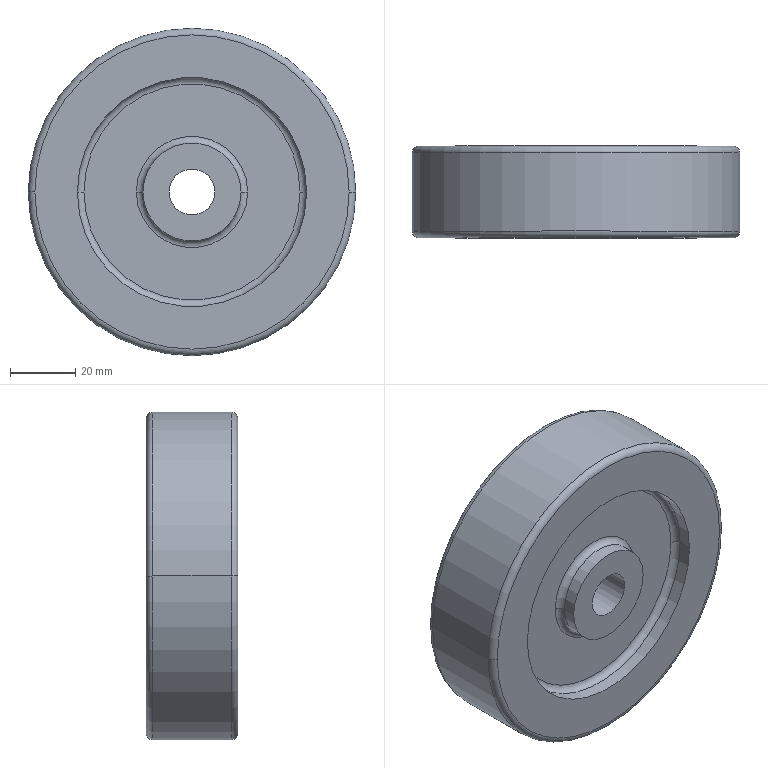Part | SolidWorks | features Fillet 2, Revolution 1 | 1 solid | 30 faces | box 100 x 28 x 100 mm | volume 177907 mm3 | torus 12 | cylinder 12 | plane 6 | commonest cylinder face diameters 30 x4 70 x4 14 x2 100 x2
STEP:
#1=CARTESIAN_POINT('',(-50.,-12.,0.));
#2=VERTEX_POINT('',#1);
#3=CARTESIAN_POINT('',(50.,-12.,0.));
#4=VERTEX_POINT('',#3);
#5=CARTESIAN_POINT('',(0.,-12.,0.));
#6=DIRECTION('',(0.,1.,0.));
#7=DIRECTION('',(1.,0.,0.));
#8=AXIS2_PLACEMENT_3D('',#5,#6,#7);
#9=CIRCLE('',#8,50.);
#10=EDGE_CURVE('',#2,#4,#9,.T.);
#11=ORIENTED_EDGE('',*,*,#10,.F.);
#12=CARTESIAN_POINT('',(-48.,-14.,0.));
#13=VERTEX_POINT('',#12);
#14=CARTESIAN_POINT('',(-48.,-12.,0.));
#15=DIRECTION('',(0.,0.,1.));
#16=DIRECTION('',(1.,0.,0.));
#17=AXIS2_PLACEMENT_3D('',#14,#15,#16);
#18=CIRCLE('',#17,2.);
#19=EDGE_CURVE('',#2,#13,#18,.T.);
#20=ORIENTED_EDGE('',*,*,#19,.T.);
#21=CARTESIAN_POINT('',(48.,-14.,0.));
#22=VERTEX_POINT('',#21);
#23=CARTESIAN_POINT('',(0.,-14.,0.));
#24=DIRECTION('',(0.,-1.,0.));
#25=DIRECTION('',(1.,0.,0.));
#26=AXIS2_PLACEMENT_3D('',#23,#24,#25);
#27=CIRCLE('',#26,48.);
#28=EDGE_CURVE('',#22,#13,#27,.T.);
#29=ORIENTED_EDGE('',*,*,#28,.F.);
#30=CARTESIAN_POINT('',(48.,-12.,0.));
#31=DIRECTION('',(0.,0.,-1.));
#32=DIRECTION('',(-1.,0.,0.));
#33=AXIS2_PLACEMENT_3D('',#30,#31,#32);
#34=CIRCLE('',#33,2.);
#35=EDGE_CURVE('',#4,#22,#34,.T.);
#36=ORIENTED_EDGE('',*,*,#35,.F.);
#37=EDGE_LOOP('',(#11,#20,#29,#36));
#38=FACE_OUTER_BOUND('',#37,.T.);
#39=CARTESIAN_POINT('',(0.,-12.,0.));
#40=DIRECTION('',(0.,-1.,0.));
#41=DIRECTION('',(1.,0.,0.));
#42=AXIS2_PLACEMENT_3D('',#39,#40,#41);
#43=TOROIDAL_SURFACE('',#42,48.,2.);
#44=ADVANCED_FACE('',(#38),#43,.T.);
#45=CARTESIAN_POINT('',(-33.,-8.,0.));
#46=VERTEX_POINT('',#45);
#47=CARTESIAN_POINT('',(33.,-8.,0.));
#48=VERTEX_POINT('',#47);
#49=CARTESIAN_POINT('',(0.,-8.,0.));
#50=DIRECTION('',(0.,-1.,0.));
#51=DIRECTION('',(1.,0.,0.));
#52=AXIS2_PLACEMENT_3D('',#49,#50,#51);
#53=CIRCLE('',#52,33.);
#54=EDGE_CURVE('',#46,#48,#53,.T.);
#55=ORIENTED_EDGE('',*,*,#54,.F.);
#56=CARTESIAN_POINT('',(-35.,-10.,0.));
#57=VERTEX_POINT('',#56);
#58=CARTESIAN_POINT('',(-33.,-10.,0.));
#59=DIRECTION('',(0.,0.,1.));
#60=DIRECTION('',(1.,0.,0.));
#61=AXIS2_PLACEMENT_3D('',#58,#59,#60);
#62=CIRCLE('',#61,2.);
#63=EDGE_CURVE('',#46,#57,#62,.T.);
#64=ORIENTED_EDGE('',*,*,#63,.T.);
#65=CARTESIAN_POINT('',(35.,-10.,0.));
#66=VERTEX_POINT('',#65);
#67=CARTESIAN_POINT('',(0.,-10.,0.));
#68=DIRECTION('',(0.,1.,0.));
#69=DIRECTION('',(1.,0.,0.));
#70=AXIS2_PLACEMENT_3D('',#67,#68,#69);
#71=CIRCLE('',#70,35.);
#72=EDGE_CURVE('',#66,#57,#71,.T.);
#73=ORIENTED_EDGE('',*,*,#72,.F.);
#74=CARTESIAN_POINT('',(33.,-10.,0.));
#75=DIRECTION('',(0.,0.,-1.));
#76=DIRECTION('',(-1.,0.,0.));
#77=AXIS2_PLACEMENT_3D('',#74,#75,#76);
#78=CIRCLE('',#77,2.);
#79=EDGE_CURVE('',#48,#66,#78,.T.);
#80=ORIENTED_EDGE('',*,*,#79,.F.);
#81=EDGE_LOOP('',(#55,#64,#73,#80));
#82=FACE_OUTER_BOUND('',#81,.T.);
#83=CARTESIAN_POINT('',(0.,-10.,0.));
#84=DIRECTION('',(0.,-1.,0.));
#85=DIRECTION('',(1.,0.,0.));
#86=AXIS2_PLACEMENT_3D('',#83,#84,#85);
#87=TOROIDAL_SURFACE('',#86,33.,2.);
#88=ADVANCED_FACE('',(#82),#87,.F.);
#89=CARTESIAN_POINT('',(-15.,-10.,0.));
#90=VERTEX_POINT('',#89);
#91=CARTESIAN_POINT('',(15.,-10.,0.));
#92=VERTEX_POINT('',#91);
#93=CARTESIAN_POINT('',(0.,-10.,0.));
#94=DIRECTION('',(0.,-1.,0.));
#95=DIRECTION('',(1.,0.,0.));
#96=AXIS2_PLACEMENT_3D('',#93,#94,#95);
#97=CIRCLE('',#96,15.);
#98=EDGE_CURVE('',#90,#92,#97,.T.);
#99=ORIENTED_EDGE('',*,*,#98,.F.);
#100=CARTESIAN_POINT('',(-17.,-8.,0.));
#101=VERTEX_POINT('',#100);
#102=CARTESIAN_POINT('',(-17.,-10.,0.));
#103=DIRECTION('',(0.,0.,1.));
#104=DIRECTION('',(1.,0.,0.));
#105=AXIS2_PLACEMENT_3D('',#102,#103,#104);
#106=CIRCLE('',#105,2.);
#107=EDGE_CURVE('',#90,#101,#106,.T.);
#108=ORIENTED_EDGE('',*,*,#107,.T.);
#109=CARTESIAN_POINT('',(17.,-8.,0.));
#110=VERTEX_POINT('',#109);
#111=CARTESIAN_POINT('',(0.,-8.,0.));
#112=DIRECTION('',(0.,1.,0.));
#113=DIRECTION('',(1.,0.,0.));
#114=AXIS2_PLACEMENT_3D('',#111,#112,#113);
#115=CIRCLE('',#114,17.);
#116=EDGE_CURVE('',#110,#101,#115,.T.);
#117=ORIENTED_EDGE('',*,*,#116,.F.);
#118=CARTESIAN_POINT('',(17.,-10.,0.));
#119=DIRECTION('',(0.,0.,-1.));
#120=DIRECTION('',(-1.,0.,0.));
#121=AXIS2_PLACEMENT_3D('',#118,#119,#120);
#122=CIRCLE('',#121,2.);
#123=EDGE_CURVE('',#92,#110,#122,.T.);
#124=ORIENTED_EDGE('',*,*,#123,.F.);
#125=EDGE_LOOP('',(#99,#108,#117,#124));
#126=FACE_OUTER_BOUND('',#125,.T.);
#127=CARTESIAN_POINT('',(0.,-10.,0.));
#128=DIRECTION('',(0.,-1.,0.));
#129=DIRECTION('',(1.,0.,0.));
#130=AXIS2_PLACEMENT_3D('',#127,#128,#129);
#131=TOROIDAL_SURFACE('',#130,17.,2.);
#132=ADVANCED_FACE('',(#126),#131,.F.);
#133=CARTESIAN_POINT('',(15.,10.,0.));
#134=VERTEX_POINT('',#133);
#135=CARTESIAN_POINT('',(-15.,10.,0.));
#136=VERTEX_POINT('',#135);
#137=CARTESIAN_POINT('',(0.,10.,0.));
#138=DIRECTION('',(0.,1.,0.));
#139=DIRECTION('',(-1.,0.,0.));
#140=AXIS2_PLACEMENT_3D('',#137,#138,#139);
#141=CIRCLE('',#140,15.);
#142=EDGE_CURVE('',#134,#136,#141,.T.);
#143=ORIENTED_EDGE('',*,*,#142,.F.);
#144=CARTESIAN_POINT('',(17.,8.,0.));
#145=VERTEX_POINT('',#144);
#146=CARTESIAN_POINT('',(17.,10.,0.));
#147=DIRECTION('',(0.,0.,1.));
#148=DIRECTION('',(1.,0.,0.));
#149=AXIS2_PLACEMENT_3D('',#146,#147,#148);
#150=CIRCLE('',#149,2.);
#151=EDGE_CURVE('',#134,#145,#150,.T.);
#152=ORIENTED_EDGE('',*,*,#151,.T.);
#153=CARTESIAN_POINT('',(-17.,8.,0.));
#154=VERTEX_POINT('',#153);
#155=CARTESIAN_POINT('',(0.,8.,0.));
#156=DIRECTION('',(0.,-1.,0.));
#157=DIRECTION('',(-1.,0.,0.));
#158=AXIS2_PLACEMENT_3D('',#155,#156,#157);
#159=CIRCLE('',#158,17.);
#160=EDGE_CURVE('',#154,#145,#159,.T.);
#161=ORIENTED_EDGE('',*,*,#160,.F.);
#162=CARTESIAN_POINT('',(-17.,10.,0.));
#163=DIRECTION('',(0.,0.,-1.));
#164=DIRECTION('',(-1.,0.,0.));
#165=AXIS2_PLACEMENT_3D('',#162,#163,#164);
#166=CIRCLE('',#165,2.);
#167=EDGE_CURVE('',#136,#154,#166,.T.);
#168=ORIENTED_EDGE('',*,*,#167,.F.);
#169=EDGE_LOOP('',(#143,#152,#161,#168));
#170=FACE_OUTER_BOUND('',#169,.T.);
#171=CARTESIAN_POINT('',(0.,10.,0.));
#172=DIRECTION('',(0.,1.,0.));
#173=DIRECTION('',(-1.,0.,0.));
#174=AXIS2_PLACEMENT_3D('',#171,#172,#173);
#175=TOROIDAL_SURFACE('',#174,17.,2.);
#176=ADVANCED_FACE('',(#170),#175,.F.);
#177=CARTESIAN_POINT('',(33.,8.,0.));
#178=VERTEX_POINT('',#177);
#179=CARTESIAN_POINT('',(-33.,8.,0.));
#180=VERTEX_POINT('',#179);
#181=CARTESIAN_POINT('',(0.,8.,0.));
#182=DIRECTION('',(0.,1.,0.));
#183=DIRECTION('',(-1.,0.,0.));
#184=AXIS2_PLACEMENT_3D('',#181,#182,#183);
#185=CIRCLE('',#184,33.);
#186=EDGE_CURVE('',#178,#180,#185,.T.);
#187=ORIENTED_EDGE('',*,*,#186,.F.);
#188=CARTESIAN_POINT('',(35.,10.,0.));
#189=VERTEX_POINT('',#188);
#190=CARTESIAN_POINT('',(33.,10.,0.));
#191=DIRECTION('',(0.,0.,1.));
#192=DIRECTION('',(1.,0.,0.));
#193=AXIS2_PLACEMENT_3D('',#190,#191,#192);
#194=CIRCLE('',#193,2.);
#195=EDGE_CURVE('',#178,#189,#194,.T.);
#196=ORIENTED_EDGE('',*,*,#195,.T.);
#197=CARTESIAN_POINT('',(-35.,10.,0.));
#198=VERTEX_POINT('',#197);
#199=CARTESIAN_POINT('',(0.,10.,0.));
#200=DIRECTION('',(0.,-1.,0.));
#201=DIRECTION('',(-1.,0.,0.));
#202=AXIS2_PLACEMENT_3D('',#199,#200,#201);
#203=CIRCLE('',#202,35.);
#204=EDGE_CURVE('',#198,#189,#203,.T.);
#205=ORIENTED_EDGE('',*,*,#204,.F.);
#206=CARTESIAN_POINT('',(-33.,10.,0.));
#207=DIRECTION('',(0.,0.,-1.));
#208=DIRECTION('',(-1.,0.,0.));
#209=AXIS2_PLACEMENT_3D('',#206,#207,#208);
#210=CIRCLE('',#209,2.);
#211=EDGE_CURVE('',#180,#198,#210,.T.);
#212=ORIENTED_EDGE('',*,*,#211,.F.);
#213=EDGE_LOOP('',(#187,#196,#205,#212));
#214=FACE_OUTER_BOUND('',#213,.T.);
#215=CARTESIAN_POINT('',(0.,10.,0.));
#216=DIRECTION('',(0.,1.,0.));
#217=DIRECTION('',(-1.,0.,0.));
#218=AXIS2_PLACEMENT_3D('',#215,#216,#217);
#219=TOROIDAL_SURFACE('',#218,33.,2.);
#220=ADVANCED_FACE('',(#214),#219,.F.);
#221=CARTESIAN_POINT('',(50.,12.,0.));
#222=VERTEX_POINT('',#221);
#223=CARTESIAN_POINT('',(-50.,12.,0.));
#224=VERTEX_POINT('',#223);
#225=CARTESIAN_POINT('',(0.,12.,0.));
#226=DIRECTION('',(0.,-1.,0.));
#227=DIRECTION('',(-1.,0.,0.));
#228=AXIS2_PLACEMENT_3D('',#225,#226,#227);
#229=CIRCLE('',#228,50.);
#230=EDGE_CURVE('',#222,#224,#229,.T.);
#231=ORIENTED_EDGE('',*,*,#230,.F.);
#232=CARTESIAN_POINT('',(48.,14.,0.));
#233=VERTEX_POINT('',#232);
#234=CARTESIAN_POINT('',(48.,12.,0.));
#235=DIRECTION('',(0.,0.,1.));
#236=DIRECTION('',(1.,0.,0.));
#237=AXIS2_PLACEMENT_3D('',#234,#235,#236);
#238=CIRCLE('',#237,2.);
#239=EDGE_CURVE('',#222,#233,#238,.T.);
#240=ORIENTED_EDGE('',*,*,#239,.T.);
#241=CARTESIAN_POINT('',(-48.,14.,0.));
#242=VERTEX_POINT('',#241);
#243=CARTESIAN_POINT('',(0.,14.,0.));
#244=DIRECTION('',(0.,1.,0.));
#245=DIRECTION('',(-1.,0.,0.));
#246=AXIS2_PLACEMENT_3D('',#243,#244,#245);
#247=CIRCLE('',#246,48.);
#248=EDGE_CURVE('',#242,#233,#247,.T.);
#249=ORIENTED_EDGE('',*,*,#248,.F.);
#250=CARTESIAN_POINT('',(-48.,12.,0.));
#251=DIRECTION('',(0.,0.,-1.));
#252=DIRECTION('',(-1.,0.,0.));
#253=AXIS2_PLACEMENT_3D('',#250,#251,#252);
#254=CIRCLE('',#253,2.);
#255=EDGE_CURVE('',#224,#242,#254,.T.);
#256=ORIENTED_EDGE('',*,*,#255,.F.);
#257=EDGE_LOOP('',(#231,#240,#249,#256));
#258=FACE_OUTER_BOUND('',#257,.T.);
#259=CARTESIAN_POINT('',(0.,12.,0.));
#260=DIRECTION('',(0.,1.,0.));
#261=DIRECTION('',(-1.,0.,0.));
#262=AXIS2_PLACEMENT_3D('',#259,#260,#261);
#263=TOROIDAL_SURFACE('',#262,48.,2.);
#264=ADVANCED_FACE('',(#258),#263,.T.);
#265=CARTESIAN_POINT('',(-7.,14.,0.));
#266=VERTEX_POINT('',#265);
#267=CARTESIAN_POINT('',(7.,14.,0.));
#268=VERTEX_POINT('',#267);
#269=CARTESIAN_POINT('',(0.,14.,0.));
#270=DIRECTION('',(0.,-1.,0.));
#271=DIRECTION('',(1.,0.,0.));
#272=AXIS2_PLACEMENT_3D('',#269,#270,#271);
#273=CIRCLE('',#272,7.);
#274=EDGE_CURVE('',#266,#268,#273,.T.);
#275=ORIENTED_EDGE('',*,*,#274,.F.);
#276=CARTESIAN_POINT('',(-7.,-14.,0.));
#277=VERTEX_POINT('',#276);
#278=CARTESIAN_POINT('',(-7.,-499.995,0.));
#279=DIRECTION('',(0.,-1.,0.));
#280=VECTOR('',#279,1000.);
#281=LINE('',#278,#280);
#282=EDGE_CURVE('',#266,#277,#281,.T.);
#283=ORIENTED_EDGE('',*,*,#282,.T.);
#284=CARTESIAN_POINT('',(7.,-14.,0.));
#285=VERTEX_POINT('',#284);
#286=CARTESIAN_POINT('',(0.,-14.,0.));
#287=DIRECTION('',(0.,-1.,0.));
#288=DIRECTION('',(1.,0.,0.));
#289=AXIS2_PLACEMENT_3D('',#286,#287,#288);
#290=CIRCLE('',#289,7.);
#291=EDGE_CURVE('',#277,#285,#290,.T.);
#292=ORIENTED_EDGE('',*,*,#291,.T.);
#293=CARTESIAN_POINT('',(7.,-499.995,0.));
#294=DIRECTION('',(0.,-1.,0.));
#295=VECTOR('',#294,1000.);
#296=LINE('',#293,#295);
#297=EDGE_CURVE('',#268,#285,#296,.T.);
#298=ORIENTED_EDGE('',*,*,#297,.F.);
#299=EDGE_LOOP('',(#275,#283,#292,#298));
#300=FACE_OUTER_BOUND('',#299,.T.);
#301=CARTESIAN_POINT('',(0.,-499.995,0.));
#302=DIRECTION('',(0.,-1.,0.));
#303=DIRECTION('',(1.,0.,0.));
#304=AXIS2_PLACEMENT_3D('',#301,#302,#303);
#305=CYLINDRICAL_SURFACE('',#304,7.);
#306=ADVANCED_FACE('',(#300),#305,.F.);
#307=CARTESIAN_POINT('',(15.,14.,0.));
#308=VERTEX_POINT('',#307);
#309=CARTESIAN_POINT('',(-15.,14.,0.));
#310=VERTEX_POINT('',#309);
#311=CARTESIAN_POINT('',(0.,14.,0.));
#312=DIRECTION('',(0.,-1.,0.));
#313=DIRECTION('',(1.,0.,0.));
#314=AXIS2_PLACEMENT_3D('',#311,#312,#313);
#315=CIRCLE('',#314,15.);
#316=EDGE_CURVE('',#308,#310,#315,.T.);
#317=ORIENTED_EDGE('',*,*,#316,.T.);
#318=CARTESIAN_POINT('',(-15.,-499.995,0.));
#319=DIRECTION('',(0.,-1.,0.));
#320=VECTOR('',#319,1000.);
#321=LINE('',#318,#320);
#322=EDGE_CURVE('',#310,#136,#321,.T.);
#323=ORIENTED_EDGE('',*,*,#322,.T.);
#324=CARTESIAN_POINT('',(0.,10.,0.));
#325=DIRECTION('',(0.,1.,0.));
#326=DIRECTION('',(-1.,0.,0.));
#327=AXIS2_PLACEMENT_3D('',#324,#325,#326);
#328=CIRCLE('',#327,15.);
#329=EDGE_CURVE('',#136,#134,#328,.T.);
#330=ORIENTED_EDGE('',*,*,#329,.T.);
#331=CARTESIAN_POINT('',(15.,-499.995,0.));
#332=DIRECTION('',(0.,-1.,0.));
#333=VECTOR('',#332,1000.);
#334=LINE('',#331,#333);
#335=EDGE_CURVE('',#308,#134,#334,.T.);
#336=ORIENTED_EDGE('',*,*,#335,.F.);
#337=EDGE_LOOP('',(#317,#323,#330,#336));
#338=FACE_OUTER_BOUND('',#337,.T.);
#339=CARTESIAN_POINT('',(0.,-499.995,0.));
#340=DIRECTION('',(0.,-1.,0.));
#341=DIRECTION('',(1.,0.,0.));
#342=AXIS2_PLACEMENT_3D('',#339,#340,#341);
#343=CYLINDRICAL_SURFACE('',#342,15.);
#344=ADVANCED_FACE('',(#338),#343,.T.);
#345=CARTESIAN_POINT('',(-35.,14.,0.));
#346=VERTEX_POINT('',#345);
#347=CARTESIAN_POINT('',(35.,14.,0.));
#348=VERTEX_POINT('',#347);
#349=CARTESIAN_POINT('',(0.,14.,0.));
#350=DIRECTION('',(0.,-1.,0.));
#351=DIRECTION('',(1.,0.,0.));
#352=AXIS2_PLACEMENT_3D('',#349,#350,#351);
#353=CIRCLE('',#352,35.);
#354=EDGE_CURVE('',#346,#348,#353,.T.);
#355=ORIENTED_EDGE('',*,*,#354,.F.);
#356=CARTESIAN_POINT('',(-35.,-499.995,0.));
#357=DIRECTION('',(0.,-1.,0.));
#358=VECTOR('',#357,1000.);
#359=LINE('',#356,#358);
#360=EDGE_CURVE('',#346,#198,#359,.T.);
#361=ORIENTED_EDGE('',*,*,#360,.T.);
#362=ORIENTED_EDGE('',*,*,#204,.T.);
#363=CARTESIAN_POINT('',(35.,-499.995,0.));
#364=DIRECTION('',(0.,-1.,0.));
#365=VECTOR('',#364,1000.);
#366=LINE('',#363,#365);
#367=EDGE_CURVE('',#348,#189,#366,.T.);
#368=ORIENTED_EDGE('',*,*,#367,.F.);
#369=EDGE_LOOP('',(#355,#361,#362,#368));
#370=FACE_OUTER_BOUND('',#369,.T.);
#371=CARTESIAN_POINT('',(0.,-499.995,0.));
#372=DIRECTION('',(0.,-1.,0.));
#373=DIRECTION('',(1.,0.,0.));
#374=AXIS2_PLACEMENT_3D('',#371,#372,#373);
#375=CYLINDRICAL_SURFACE('',#374,35.);
#376=ADVANCED_FACE('',(#370),#375,.F.);
#377=ORIENTED_EDGE('',*,*,#230,.T.);
#378=CARTESIAN_POINT('',(-50.,-499.995,0.));
#379=DIRECTION('',(0.,-1.,0.));
#380=VECTOR('',#379,1000.);
#381=LINE('',#378,#380);
#382=EDGE_CURVE('',#224,#2,#381,.T.);
#383=ORIENTED_EDGE('',*,*,#382,.T.);
#384=ORIENTED_EDGE('',*,*,#10,.T.);
#385=CARTESIAN_POINT('',(50.,-499.995,0.));
#386=DIRECTION('',(0.,-1.,0.));
#387=VECTOR('',#386,1000.);
#388=LINE('',#385,#387);
#389=EDGE_CURVE('',#222,#4,#388,.T.);
#390=ORIENTED_EDGE('',*,*,#389,.F.);
#391=EDGE_LOOP('',(#377,#383,#384,#390));
#392=FACE_OUTER_BOUND('',#391,.T.);
#393=CARTESIAN_POINT('',(0.,-499.995,0.));
#394=DIRECTION('',(0.,-1.,0.));
#395=DIRECTION('',(1.,0.,0.));
#396=AXIS2_PLACEMENT_3D('',#393,#394,#395);
#397=CYLINDRICAL_SURFACE('',#396,50.);
#398=ADVANCED_FACE('',(#392),#397,.T.);
#399=ORIENTED_EDGE('',*,*,#72,.T.);
#400=CARTESIAN_POINT('',(-35.,-14.,0.));
#401=VERTEX_POINT('',#400);
#402=CARTESIAN_POINT('',(-35.,-499.995,0.));
#403=DIRECTION('',(0.,-1.,0.));
#404=VECTOR('',#403,1000.);
#405=LINE('',#402,#404);
#406=EDGE_CURVE('',#57,#401,#405,.T.);
#407=ORIENTED_EDGE('',*,*,#406,.T.);
#408=CARTESIAN_POINT('',(35.,-14.,0.));
#409=VERTEX_POINT('',#408);
#410=CARTESIAN_POINT('',(0.,-14.,0.));
#411=DIRECTION('',(0.,-1.,0.));
#412=DIRECTION('',(1.,0.,0.));
#413=AXIS2_PLACEMENT_3D('',#410,#411,#412);
#414=CIRCLE('',#413,35.);
#415=EDGE_CURVE('',#401,#409,#414,.T.);
#416=ORIENTED_EDGE('',*,*,#415,.T.);
#417=CARTESIAN_POINT('',(35.,-499.995,0.));
#418=DIRECTION('',(0.,-1.,0.));
#419=VECTOR('',#418,1000.);
#420=LINE('',#417,#419);
#421=EDGE_CURVE('',#66,#409,#420,.T.);
#422=ORIENTED_EDGE('',*,*,#421,.F.);
#423=EDGE_LOOP('',(#399,#407,#416,#422));
#424=FACE_OUTER_BOUND('',#423,.T.);
#425=CARTESIAN_POINT('',(0.,-499.995,0.));
#426=DIRECTION('',(0.,-1.,0.));
#427=DIRECTION('',(1.,0.,0.));
#428=AXIS2_PLACEMENT_3D('',#425,#426,#427);
#429=CYLINDRICAL_SURFACE('',#428,35.);
#430=ADVANCED_FACE('',(#424),#429,.F.);
#431=CARTESIAN_POINT('',(0.,-10.,0.));
#432=DIRECTION('',(0.,-1.,0.));
#433=DIRECTION('',(1.,0.,0.));
#434=AXIS2_PLACEMENT_3D('',#431,#432,#433);
#435=CIRCLE('',#434,15.);
#436=EDGE_CURVE('',#92,#90,#435,.T.);
#437=ORIENTED_EDGE('',*,*,#436,.T.);
#438=CARTESIAN_POINT('',(-15.,-14.,0.));
#439=VERTEX_POINT('',#438);
#440=CARTESIAN_POINT('',(-15.,-499.995,0.));
#441=DIRECTION('',(0.,-1.,0.));
#442=VECTOR('',#441,1000.);
#443=LINE('',#440,#442);
#444=EDGE_CURVE('',#90,#439,#443,.T.);
#445=ORIENTED_EDGE('',*,*,#444,.T.);
#446=CARTESIAN_POINT('',(15.,-14.,0.));
#447=VERTEX_POINT('',#446);
#448=CARTESIAN_POINT('',(0.,-14.,0.));
#449=DIRECTION('',(0.,-1.,0.));
#450=DIRECTION('',(1.,0.,0.));
#451=AXIS2_PLACEMENT_3D('',#448,#449,#450);
#452=CIRCLE('',#451,15.);
#453=EDGE_CURVE('',#447,#439,#452,.T.);
#454=ORIENTED_EDGE('',*,*,#453,.F.);
#455=CARTESIAN_POINT('',(15.,-499.995,0.));
#456=DIRECTION('',(0.,-1.,0.));
#457=VECTOR('',#456,1000.);
#458=LINE('',#455,#457);
#459=EDGE_CURVE('',#92,#447,#458,.T.);
#460=ORIENTED_EDGE('',*,*,#459,.F.);
#461=EDGE_LOOP('',(#437,#445,#454,#460));
#462=FACE_OUTER_BOUND('',#461,.T.);
#463=CARTESIAN_POINT('',(0.,-499.995,0.));
#464=DIRECTION('',(0.,-1.,0.));
#465=DIRECTION('',(1.,0.,0.));
#466=AXIS2_PLACEMENT_3D('',#463,#464,#465);
#467=CYLINDRICAL_SURFACE('',#466,15.);
#468=ADVANCED_FACE('',(#462),#467,.T.);
#469=ORIENTED_EDGE('',*,*,#444,.F.);
#470=ORIENTED_EDGE('',*,*,#98,.T.);
#471=ORIENTED_EDGE('',*,*,#459,.T.);
#472=CARTESIAN_POINT('',(0.,-14.,0.));
#473=DIRECTION('',(0.,-1.,0.));
#474=DIRECTION('',(1.,0.,0.));
#475=AXIS2_PLACEMENT_3D('',#472,#473,#474);
#476=CIRCLE('',#475,15.);
#477=EDGE_CURVE('',#439,#447,#476,.T.);
#478=ORIENTED_EDGE('',*,*,#477,.F.);
#479=EDGE_LOOP('',(#469,#470,#471,#478));
#480=FACE_OUTER_BOUND('',#479,.T.);
#481=CARTESIAN_POINT('',(0.,-499.995,0.));
#482=DIRECTION('',(0.,-1.,0.));
#483=DIRECTION('',(1.,0.,0.));
#484=AXIS2_PLACEMENT_3D('',#481,#482,#483);
#485=CYLINDRICAL_SURFACE('',#484,15.);
#486=ADVANCED_FACE('',(#480),#485,.T.);
#487=ORIENTED_EDGE('',*,*,#116,.T.);
#488=CARTESIAN_POINT('',(0.,-8.,0.));
#489=DIRECTION('',(0.,1.,0.));
#490=DIRECTION('',(1.,0.,0.));
#491=AXIS2_PLACEMENT_3D('',#488,#489,#490);
#492=CIRCLE('',#491,17.);
#493=EDGE_CURVE('',#101,#110,#492,.T.);
#494=ORIENTED_EDGE('',*,*,#493,.T.);
#495=EDGE_LOOP('',(#487,#494));
#496=FACE_BOUND('',#495,.T.);
#497=CARTESIAN_POINT('',(0.,-8.,0.));
#498=DIRECTION('',(0.,-1.,0.));
#499=DIRECTION('',(1.,0.,0.));
#500=AXIS2_PLACEMENT_3D('',#497,#498,#499);
#501=CIRCLE('',#500,33.);
#502=EDGE_CURVE('',#48,#46,#501,.T.);
#503=ORIENTED_EDGE('',*,*,#502,.T.);
#504=ORIENTED_EDGE('',*,*,#54,.T.);
#505=EDGE_LOOP('',(#503,#504));
#506=FACE_OUTER_BOUND('',#505,.T.);
#507=CARTESIAN_POINT('',(35.,-8.,0.));
#508=DIRECTION('',(0.,-1.,0.));
#509=DIRECTION('',(1.,0.,0.));
#510=AXIS2_PLACEMENT_3D('',#507,#508,#509);
#511=PLANE('',#510);
#512=ADVANCED_FACE('',(#496,#506),#511,.T.);
#513=ORIENTED_EDGE('',*,*,#406,.F.);
#514=CARTESIAN_POINT('',(0.,-10.,0.));
#515=DIRECTION('',(0.,1.,0.));
#516=DIRECTION('',(1.,0.,0.));
#517=AXIS2_PLACEMENT_3D('',#514,#515,#516);
#518=CIRCLE('',#517,35.);
#519=EDGE_CURVE('',#57,#66,#518,.T.);
#520=ORIENTED_EDGE('',*,*,#519,.T.);
#521=ORIENTED_EDGE('',*,*,#421,.T.);
#522=CARTESIAN_POINT('',(0.,-14.,0.));
#523=DIRECTION('',(0.,-1.,0.));
#524=DIRECTION('',(1.,0.,0.));
#525=AXIS2_PLACEMENT_3D('',#522,#523,#524);
#526=CIRCLE('',#525,35.);
#527=EDGE_CURVE('',#409,#401,#526,.T.);
#528=ORIENTED_EDGE('',*,*,#527,.T.);
#529=EDGE_LOOP('',(#513,#520,#521,#528));
#530=FACE_OUTER_BOUND('',#529,.T.);
#531=CARTESIAN_POINT('',(0.,-499.995,0.));
#532=DIRECTION('',(0.,-1.,0.));
#533=DIRECTION('',(1.,0.,0.));
#534=AXIS2_PLACEMENT_3D('',#531,#532,#533);
#535=CYLINDRICAL_SURFACE('',#534,35.);
#536=ADVANCED_FACE('',(#530),#535,.F.);
#537=ORIENTED_EDGE('',*,*,#28,.T.);
#538=CARTESIAN_POINT('',(0.,-14.,0.));
#539=DIRECTION('',(0.,-1.,0.));
#540=DIRECTION('',(1.,0.,0.));
#541=AXIS2_PLACEMENT_3D('',#538,#539,#540);
#542=CIRCLE('',#541,48.);
#543=EDGE_CURVE('',#13,#22,#542,.T.);
#544=ORIENTED_EDGE('',*,*,#543,.T.);
#545=EDGE_LOOP('',(#537,#544));
#546=FACE_OUTER_BOUND('',#545,.T.);
#547=ORIENTED_EDGE('',*,*,#527,.F.);
#548=ORIENTED_EDGE('',*,*,#415,.F.);
#549=EDGE_LOOP('',(#547,#548));
#550=FACE_BOUND('',#549,.T.);
#551=CARTESIAN_POINT('',(50.,-14.,0.));
#552=DIRECTION('',(0.,-1.,0.));
#553=DIRECTION('',(1.,0.,0.));
#554=AXIS2_PLACEMENT_3D('',#551,#552,#553);
#555=PLANE('',#554);
#556=ADVANCED_FACE('',(#546,#550),#555,.T.);
#557=ORIENTED_EDGE('',*,*,#382,.F.);
#558=CARTESIAN_POINT('',(0.,12.,0.));
#559=DIRECTION('',(0.,-1.,0.));
#560=DIRECTION('',(-1.,0.,0.));
#561=AXIS2_PLACEMENT_3D('',#558,#559,#560);
#562=CIRCLE('',#561,50.);
#563=EDGE_CURVE('',#224,#222,#562,.T.);
#564=ORIENTED_EDGE('',*,*,#563,.T.);
#565=ORIENTED_EDGE('',*,*,#389,.T.);
#566=CARTESIAN_POINT('',(0.,-12.,0.));
#567=DIRECTION('',(0.,1.,0.));
#568=DIRECTION('',(1.,0.,0.));
#569=AXIS2_PLACEMENT_3D('',#566,#567,#568);
#570=CIRCLE('',#569,50.);
#571=EDGE_CURVE('',#4,#2,#570,.T.);
#572=ORIENTED_EDGE('',*,*,#571,.T.);
#573=EDGE_LOOP('',(#557,#564,#565,#572));
#574=FACE_OUTER_BOUND('',#573,.T.);
#575=CARTESIAN_POINT('',(0.,-499.995,0.));
#576=DIRECTION('',(0.,-1.,0.));
#577=DIRECTION('',(1.,0.,0.));
#578=AXIS2_PLACEMENT_3D('',#575,#576,#577);
#579=CYLINDRICAL_SURFACE('',#578,50.);
#580=ADVANCED_FACE('',(#574),#579,.T.);
#581=ORIENTED_EDGE('',*,*,#248,.T.);
#582=CARTESIAN_POINT('',(0.,14.,0.));
#583=DIRECTION('',(0.,1.,0.));
#584=DIRECTION('',(-1.,0.,0.));
#585=AXIS2_PLACEMENT_3D('',#582,#583,#584);
#586=CIRCLE('',#585,48.);
#587=EDGE_CURVE('',#233,#242,#586,.T.);
#588=ORIENTED_EDGE('',*,*,#587,.T.);
#589=EDGE_LOOP('',(#581,#588));
#590=FACE_OUTER_BOUND('',#589,.T.);
#591=CARTESIAN_POINT('',(0.,14.,0.));
#592=DIRECTION('',(0.,-1.,0.));
#593=DIRECTION('',(1.,0.,0.));
#594=AXIS2_PLACEMENT_3D('',#591,#592,#593);
#595=CIRCLE('',#594,35.);
#596=EDGE_CURVE('',#348,#346,#595,.T.);
#597=ORIENTED_EDGE('',*,*,#596,.T.);
#598=ORIENTED_EDGE('',*,*,#354,.T.);
#599=EDGE_LOOP('',(#597,#598));
#600=FACE_BOUND('',#599,.T.);
#601=CARTESIAN_POINT('',(35.,14.,0.));
#602=DIRECTION('',(0.,1.,0.));
#603=DIRECTION('',(-1.,0.,0.));
#604=AXIS2_PLACEMENT_3D('',#601,#602,#603);
#605=PLANE('',#604);
#606=ADVANCED_FACE('',(#590,#600),#605,.T.);
#607=ORIENTED_EDGE('',*,*,#360,.F.);
#608=ORIENTED_EDGE('',*,*,#596,.F.);
#609=ORIENTED_EDGE('',*,*,#367,.T.);
#610=CARTESIAN_POINT('',(0.,10.,0.));
#611=DIRECTION('',(0.,-1.,0.));
#612=DIRECTION('',(-1.,0.,0.));
#613=AXIS2_PLACEMENT_3D('',#610,#611,#612);
#614=CIRCLE('',#613,35.);
#615=EDGE_CURVE('',#189,#198,#614,.T.);
#616=ORIENTED_EDGE('',*,*,#615,.T.);
#617=EDGE_LOOP('',(#607,#608,#609,#616));
#618=FACE_OUTER_BOUND('',#617,.T.);
#619=CARTESIAN_POINT('',(0.,-499.995,0.));
#620=DIRECTION('',(0.,-1.,0.));
#621=DIRECTION('',(1.,0.,0.));
#622=AXIS2_PLACEMENT_3D('',#619,#620,#621);
#623=CYLINDRICAL_SURFACE('',#622,35.);
#624=ADVANCED_FACE('',(#618),#623,.F.);
#625=CARTESIAN_POINT('',(0.,8.,0.));
#626=DIRECTION('',(0.,1.,0.));
#627=DIRECTION('',(-1.,0.,0.));
#628=AXIS2_PLACEMENT_3D('',#625,#626,#627);
#629=CIRCLE('',#628,33.);
#630=EDGE_CURVE('',#180,#178,#629,.T.);
#631=ORIENTED_EDGE('',*,*,#630,.T.);
#632=ORIENTED_EDGE('',*,*,#186,.T.);
#633=EDGE_LOOP('',(#631,#632));
#634=FACE_OUTER_BOUND('',#633,.T.);
#635=ORIENTED_EDGE('',*,*,#160,.T.);
#636=CARTESIAN_POINT('',(0.,8.,0.));
#637=DIRECTION('',(0.,-1.,0.));
#638=DIRECTION('',(-1.,0.,0.));
#639=AXIS2_PLACEMENT_3D('',#636,#637,#638);
#640=CIRCLE('',#639,17.);
#641=EDGE_CURVE('',#145,#154,#640,.T.);
#642=ORIENTED_EDGE('',*,*,#641,.T.);
#643=EDGE_LOOP('',(#635,#642));
#644=FACE_BOUND('',#643,.T.);
#645=CARTESIAN_POINT('',(15.,8.,0.));
#646=DIRECTION('',(0.,1.,0.));
#647=DIRECTION('',(-1.,0.,0.));
#648=AXIS2_PLACEMENT_3D('',#645,#646,#647);
#649=PLANE('',#648);
#650=ADVANCED_FACE('',(#634,#644),#649,.T.);
#651=ORIENTED_EDGE('',*,*,#322,.F.);
#652=CARTESIAN_POINT('',(0.,14.,0.));
#653=DIRECTION('',(0.,-1.,0.));
#654=DIRECTION('',(1.,0.,0.));
#655=AXIS2_PLACEMENT_3D('',#652,#653,#654);
#656=CIRCLE('',#655,15.);
#657=EDGE_CURVE('',#310,#308,#656,.T.);
#658=ORIENTED_EDGE('',*,*,#657,.T.);
#659=ORIENTED_EDGE('',*,*,#335,.T.);
#660=ORIENTED_EDGE('',*,*,#142,.T.);
#661=EDGE_LOOP('',(#651,#658,#659,#660));
#662=FACE_OUTER_BOUND('',#661,.T.);
#663=CARTESIAN_POINT('',(0.,-499.995,0.));
#664=DIRECTION('',(0.,-1.,0.));
#665=DIRECTION('',(1.,0.,0.));
#666=AXIS2_PLACEMENT_3D('',#663,#664,#665);
#667=CYLINDRICAL_SURFACE('',#666,15.);
#668=ADVANCED_FACE('',(#662),#667,.T.);
#669=CARTESIAN_POINT('',(0.,14.,0.));
#670=DIRECTION('',(0.,-1.,0.));
#671=DIRECTION('',(1.,0.,0.));
#672=AXIS2_PLACEMENT_3D('',#669,#670,#671);
#673=CIRCLE('',#672,7.);
#674=EDGE_CURVE('',#268,#266,#673,.T.);
#675=ORIENTED_EDGE('',*,*,#674,.T.);
#676=ORIENTED_EDGE('',*,*,#274,.T.);
#677=EDGE_LOOP('',(#675,#676));
#678=FACE_BOUND('',#677,.T.);
#679=ORIENTED_EDGE('',*,*,#316,.F.);
#680=ORIENTED_EDGE('',*,*,#657,.F.);
#681=EDGE_LOOP('',(#679,#680));
#682=FACE_OUTER_BOUND('',#681,.T.);
#683=CARTESIAN_POINT('',(7.,14.,0.));
#684=DIRECTION('',(0.,1.,0.));
#685=DIRECTION('',(-1.,0.,0.));
#686=AXIS2_PLACEMENT_3D('',#683,#684,#685);
#687=PLANE('',#686);
#688=ADVANCED_FACE('',(#678,#682),#687,.T.);
#689=ORIENTED_EDGE('',*,*,#282,.F.);
#690=ORIENTED_EDGE('',*,*,#674,.F.);
#691=ORIENTED_EDGE('',*,*,#297,.T.);
#692=CARTESIAN_POINT('',(0.,-14.,0.));
#693=DIRECTION('',(0.,-1.,0.));
#694=DIRECTION('',(1.,0.,0.));
#695=AXIS2_PLACEMENT_3D('',#692,#693,#694);
#696=CIRCLE('',#695,7.);
#697=EDGE_CURVE('',#285,#277,#696,.T.);
#698=ORIENTED_EDGE('',*,*,#697,.T.);
#699=EDGE_LOOP('',(#689,#690,#691,#698));
#700=FACE_OUTER_BOUND('',#699,.T.);
#701=CARTESIAN_POINT('',(0.,-499.995,0.));
#702=DIRECTION('',(0.,-1.,0.));
#703=DIRECTION('',(1.,0.,0.));
#704=AXIS2_PLACEMENT_3D('',#701,#702,#703);
#705=CYLINDRICAL_SURFACE('',#704,7.);
#706=ADVANCED_FACE('',(#700),#705,.F.);
#707=ORIENTED_EDGE('',*,*,#453,.T.);
#708=ORIENTED_EDGE('',*,*,#477,.T.);
#709=EDGE_LOOP('',(#707,#708));
#710=FACE_OUTER_BOUND('',#709,.T.);
#711=ORIENTED_EDGE('',*,*,#697,.F.);
#712=ORIENTED_EDGE('',*,*,#291,.F.);
#713=EDGE_LOOP('',(#711,#712));
#714=FACE_BOUND('',#713,.T.);
#715=CARTESIAN_POINT('',(7.,-14.,0.));
#716=DIRECTION('',(0.,-1.,0.));
#717=DIRECTION('',(1.,0.,0.));
#718=AXIS2_PLACEMENT_3D('',#715,#716,#717);
#719=PLANE('',#718);
#720=ADVANCED_FACE('',(#710,#714),#719,.T.);
#721=ORIENTED_EDGE('',*,*,#239,.F.);
#722=ORIENTED_EDGE('',*,*,#563,.F.);
#723=ORIENTED_EDGE('',*,*,#255,.T.);
#724=ORIENTED_EDGE('',*,*,#587,.F.);
#725=EDGE_LOOP('',(#721,#722,#723,#724));
#726=FACE_OUTER_BOUND('',#725,.T.);
#727=CARTESIAN_POINT('',(0.,12.,0.));
#728=DIRECTION('',(0.,1.,0.));
#729=DIRECTION('',(-1.,0.,0.));
#730=AXIS2_PLACEMENT_3D('',#727,#728,#729);
#731=TOROIDAL_SURFACE('',#730,48.,2.);
#732=ADVANCED_FACE('',(#726),#731,.T.);
#733=ORIENTED_EDGE('',*,*,#195,.F.);
#734=ORIENTED_EDGE('',*,*,#630,.F.);
#735=ORIENTED_EDGE('',*,*,#211,.T.);
#736=ORIENTED_EDGE('',*,*,#615,.F.);
#737=EDGE_LOOP('',(#733,#734,#735,#736));
#738=FACE_OUTER_BOUND('',#737,.T.);
#739=CARTESIAN_POINT('',(0.,10.,0.));
#740=DIRECTION('',(0.,1.,0.));
#741=DIRECTION('',(-1.,0.,0.));
#742=AXIS2_PLACEMENT_3D('',#739,#740,#741);
#743=TOROIDAL_SURFACE('',#742,33.,2.);
#744=ADVANCED_FACE('',(#738),#743,.F.);
#745=ORIENTED_EDGE('',*,*,#151,.F.);
#746=ORIENTED_EDGE('',*,*,#329,.F.);
#747=ORIENTED_EDGE('',*,*,#167,.T.);
#748=ORIENTED_EDGE('',*,*,#641,.F.);
#749=EDGE_LOOP('',(#745,#746,#747,#748));
#750=FACE_OUTER_BOUND('',#749,.T.);
#751=CARTESIAN_POINT('',(0.,10.,0.));
#752=DIRECTION('',(0.,1.,0.));
#753=DIRECTION('',(-1.,0.,0.));
#754=AXIS2_PLACEMENT_3D('',#751,#752,#753);
#755=TOROIDAL_SURFACE('',#754,17.,2.);
#756=ADVANCED_FACE('',(#750),#755,.F.);
#757=ORIENTED_EDGE('',*,*,#107,.F.);
#758=ORIENTED_EDGE('',*,*,#436,.F.);
#759=ORIENTED_EDGE('',*,*,#123,.T.);
#760=ORIENTED_EDGE('',*,*,#493,.F.);
#761=EDGE_LOOP('',(#757,#758,#759,#760));
#762=FACE_OUTER_BOUND('',#761,.T.);
#763=CARTESIAN_POINT('',(0.,-10.,0.));
#764=DIRECTION('',(0.,-1.,0.));
#765=DIRECTION('',(1.,0.,0.));
#766=AXIS2_PLACEMENT_3D('',#763,#764,#765);
#767=TOROIDAL_SURFACE('',#766,17.,2.);
#768=ADVANCED_FACE('',(#762),#767,.F.);
#769=ORIENTED_EDGE('',*,*,#63,.F.);
#770=ORIENTED_EDGE('',*,*,#502,.F.);
#771=ORIENTED_EDGE('',*,*,#79,.T.);
#772=ORIENTED_EDGE('',*,*,#519,.F.);
#773=EDGE_LOOP('',(#769,#770,#771,#772));
#774=FACE_OUTER_BOUND('',#773,.T.);
#775=CARTESIAN_POINT('',(0.,-10.,0.));
#776=DIRECTION('',(0.,-1.,0.));
#777=DIRECTION('',(1.,0.,0.));
#778=AXIS2_PLACEMENT_3D('',#775,#776,#777);
#779=TOROIDAL_SURFACE('',#778,33.,2.);
#780=ADVANCED_FACE('',(#774),#779,.F.);
#781=ORIENTED_EDGE('',*,*,#19,.F.);
#782=ORIENTED_EDGE('',*,*,#571,.F.);
#783=ORIENTED_EDGE('',*,*,#35,.T.);
#784=ORIENTED_EDGE('',*,*,#543,.F.);
#785=EDGE_LOOP('',(#781,#782,#783,#784));
#786=FACE_OUTER_BOUND('',#785,.T.);
#787=CARTESIAN_POINT('',(0.,-12.,0.));
#788=DIRECTION('',(0.,-1.,0.));
#789=DIRECTION('',(1.,0.,0.));
#790=AXIS2_PLACEMENT_3D('',#787,#788,#789);
#791=TOROIDAL_SURFACE('',#790,48.,2.);
#792=ADVANCED_FACE('',(#786),#791,.T.);
#793=CLOSED_SHELL('',(#44,#88,#132,#176,#220,#264,#306,#344,#376,#398,#430,#468,#486,#512,#536,#556,#580,#606,#624,#650,#668,#688,#706,#720,#732,#744,#756,#768,#780,#792));
#794=MANIFOLD_SOLID_BREP('',#793);
#795=CARTESIAN_POINT('',(0.,0.,0.));
#796=DIRECTION('',(0.,0.,1.));
#797=DIRECTION('',(1.,0.,0.));
#798=AXIS2_PLACEMENT_3D('',#795,#796,#797);
#799=(LENGTH_UNIT()NAMED_UNIT(*)SI_UNIT(.MILLI.,.METRE.));
#800=UNCERTAINTY_MEASURE_WITH_UNIT(LENGTH_MEASURE(0.00001),#799,'','');
#801=(NAMED_UNIT(*)PLANE_ANGLE_UNIT()SI_UNIT($,.RADIAN.));
#802=(NAMED_UNIT(*)SI_UNIT($,.STERADIAN.)SOLID_ANGLE_UNIT());
#803=(GEOMETRIC_REPRESENTATION_CONTEXT(3)GLOBAL_UNCERTAINTY_ASSIGNED_CONTEXT((#800))GLOBAL_UNIT_ASSIGNED_CONTEXT((#799,#801,#802))REPRESENTATION_CONTEXT('',''));
#804=ADVANCED_BREP_SHAPE_REPRESENTATION('',(#794,#798),#803);